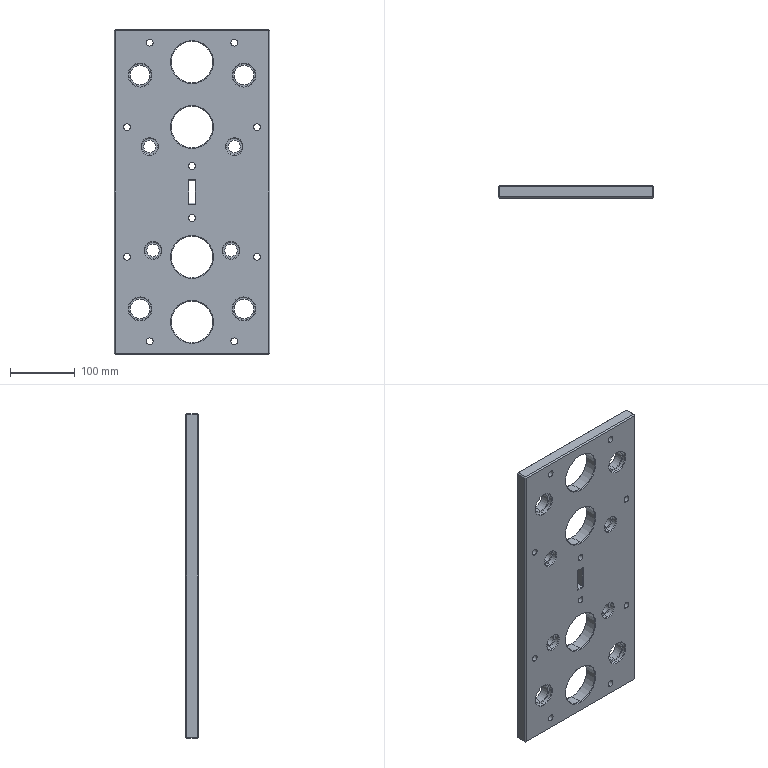Part | STEP file | PE - Torre - 1 cav | 1 solid | 154 faces | box 240 x 20 x 500 mm | volume 2018686 mm3 | cylinder 60 | cone 48 | plane 46 | commonest cylinder face diameters 10.5 x20 19 x8 25 x8 30 x8 35 x8 64 x8